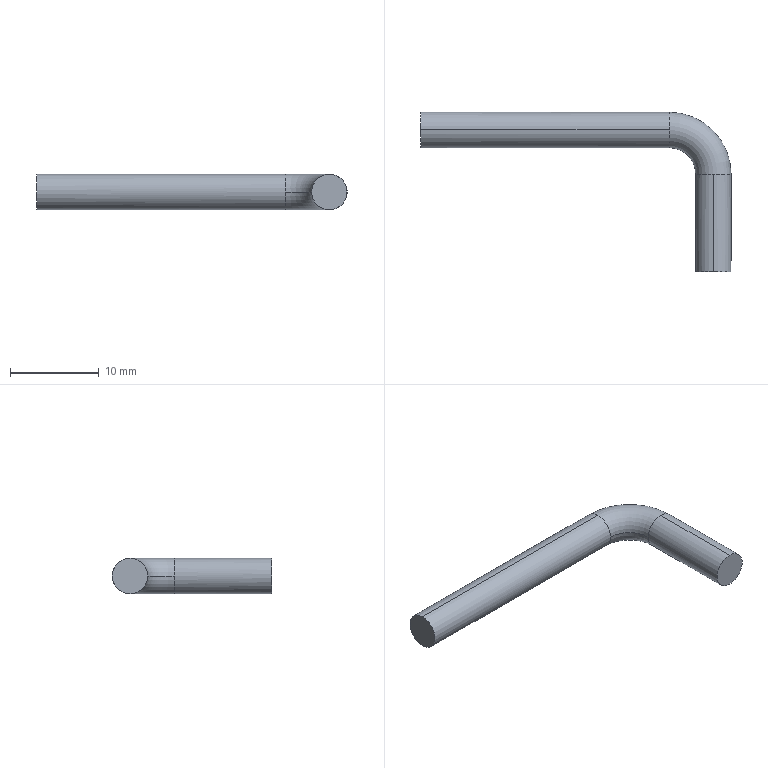Part | SolidWorks | features Sweep 1 | 1 solid | 8 faces | box 35 x 18 x 4 mm | volume 588.784 mm3 | cylinder 4 | torus 2 | plane 2 | commonest cylinder face diameters 4 x4
STEP:
#1=CARTESIAN_POINT('',(28.,2.,0.));
#2=VERTEX_POINT('',#1);
#3=CARTESIAN_POINT('',(28.,0.,-2.));
#4=VERTEX_POINT('',#3);
#5=CARTESIAN_POINT('',(28.,0.,0.));
#6=DIRECTION('',(-1.,0.,0.));
#7=DIRECTION('',(0.,0.,1.));
#8=AXIS2_PLACEMENT_3D('',#5,#6,#7);
#9=CIRCLE('',#8,2.);
#10=EDGE_CURVE('',#2,#4,#9,.T.);
#11=ORIENTED_EDGE('',*,*,#10,.F.);
#12=CARTESIAN_POINT('',(35.,-5.,0.));
#13=VERTEX_POINT('',#12);
#14=CARTESIAN_POINT('',(28.,-5.,0.));
#15=DIRECTION('',(0.,0.,-1.));
#16=DIRECTION('',(-1.,0.,0.));
#17=AXIS2_PLACEMENT_3D('',#14,#15,#16);
#18=CIRCLE('',#17,7.);
#19=EDGE_CURVE('',#2,#13,#18,.T.);
#20=ORIENTED_EDGE('',*,*,#19,.T.);
#21=CARTESIAN_POINT('',(33.,-5.,-2.));
#22=VERTEX_POINT('',#21);
#23=CARTESIAN_POINT('',(33.,-5.,0.));
#24=DIRECTION('',(0.,1.,0.));
#25=DIRECTION('',(0.,0.,1.));
#26=AXIS2_PLACEMENT_3D('',#23,#24,#25);
#27=CIRCLE('',#26,2.);
#28=EDGE_CURVE('',#13,#22,#27,.T.);
#29=ORIENTED_EDGE('',*,*,#28,.T.);
#30=CARTESIAN_POINT('',(31.,-5.,0.));
#31=VERTEX_POINT('',#30);
#32=CARTESIAN_POINT('',(33.,-5.,0.));
#33=DIRECTION('',(0.,1.,0.));
#34=DIRECTION('',(0.,0.,1.));
#35=AXIS2_PLACEMENT_3D('',#32,#33,#34);
#36=CIRCLE('',#35,2.);
#37=EDGE_CURVE('',#22,#31,#36,.T.);
#38=ORIENTED_EDGE('',*,*,#37,.T.);
#39=CARTESIAN_POINT('',(28.,-2.,0.));
#40=VERTEX_POINT('',#39);
#41=CARTESIAN_POINT('',(28.,-5.,0.));
#42=DIRECTION('',(0.,0.,-1.));
#43=DIRECTION('',(-1.,0.,0.));
#44=AXIS2_PLACEMENT_3D('',#41,#42,#43);
#45=CIRCLE('',#44,3.);
#46=EDGE_CURVE('',#40,#31,#45,.T.);
#47=ORIENTED_EDGE('',*,*,#46,.F.);
#48=CARTESIAN_POINT('',(28.,0.,0.));
#49=DIRECTION('',(-1.,0.,0.));
#50=DIRECTION('',(0.,0.,1.));
#51=AXIS2_PLACEMENT_3D('',#48,#49,#50);
#52=CIRCLE('',#51,2.);
#53=EDGE_CURVE('',#4,#40,#52,.T.);
#54=ORIENTED_EDGE('',*,*,#53,.F.);
#55=EDGE_LOOP('',(#11,#20,#29,#38,#47,#54));
#56=FACE_OUTER_BOUND('',#55,.T.);
#57=CARTESIAN_POINT('',(28.,-5.,0.));
#58=DIRECTION('',(0.,0.,-1.));
#59=DIRECTION('',(-1.,0.,0.));
#60=AXIS2_PLACEMENT_3D('',#57,#58,#59);
#61=TOROIDAL_SURFACE('',#60,5.,2.);
#62=ADVANCED_FACE('',(#56),#61,.T.);
#63=CARTESIAN_POINT('',(33.,-5.,2.));
#64=VERTEX_POINT('',#63);
#65=CARTESIAN_POINT('',(33.,-5.,0.));
#66=DIRECTION('',(0.,1.,0.));
#67=DIRECTION('',(0.,0.,1.));
#68=AXIS2_PLACEMENT_3D('',#65,#66,#67);
#69=CIRCLE('',#68,2.);
#70=EDGE_CURVE('',#64,#13,#69,.T.);
#71=ORIENTED_EDGE('',*,*,#70,.F.);
#72=CARTESIAN_POINT('',(33.,-16.,2.));
#73=VERTEX_POINT('',#72);
#74=CARTESIAN_POINT('',(33.,-5.,2.));
#75=DIRECTION('',(0.,-1.,0.));
#76=VECTOR('',#75,1000.);
#77=LINE('',#74,#76);
#78=EDGE_CURVE('',#64,#73,#77,.T.);
#79=ORIENTED_EDGE('',*,*,#78,.T.);
#80=CARTESIAN_POINT('',(33.,-16.,-2.));
#81=VERTEX_POINT('',#80);
#82=CARTESIAN_POINT('',(33.,-16.,0.));
#83=DIRECTION('',(0.,1.,0.));
#84=DIRECTION('',(0.,0.,1.));
#85=AXIS2_PLACEMENT_3D('',#82,#83,#84);
#86=CIRCLE('',#85,2.);
#87=EDGE_CURVE('',#73,#81,#86,.T.);
#88=ORIENTED_EDGE('',*,*,#87,.T.);
#89=CARTESIAN_POINT('',(33.,-5.,-2.));
#90=DIRECTION('',(0.,-1.,0.));
#91=VECTOR('',#90,1000.);
#92=LINE('',#89,#91);
#93=EDGE_CURVE('',#22,#81,#92,.T.);
#94=ORIENTED_EDGE('',*,*,#93,.F.);
#95=ORIENTED_EDGE('',*,*,#28,.F.);
#96=EDGE_LOOP('',(#71,#79,#88,#94,#95));
#97=FACE_OUTER_BOUND('',#96,.T.);
#98=CARTESIAN_POINT('',(33.,-5.,0.));
#99=DIRECTION('',(0.,-1.,0.));
#100=DIRECTION('',(0.,0.,-1.));
#101=AXIS2_PLACEMENT_3D('',#98,#99,#100);
#102=CYLINDRICAL_SURFACE('',#101,2.);
#103=ADVANCED_FACE('',(#97),#102,.T.);
#104=CARTESIAN_POINT('',(0.,0.,2.));
#105=VERTEX_POINT('',#104);
#106=CARTESIAN_POINT('',(0.,0.,-2.));
#107=VERTEX_POINT('',#106);
#108=CARTESIAN_POINT('',(0.,0.,0.));
#109=DIRECTION('',(-1.,0.,0.));
#110=DIRECTION('',(0.,0.,1.));
#111=AXIS2_PLACEMENT_3D('',#108,#109,#110);
#112=CIRCLE('',#111,2.);
#113=EDGE_CURVE('',#105,#107,#112,.T.);
#114=ORIENTED_EDGE('',*,*,#113,.F.);
#115=CARTESIAN_POINT('',(28.,0.,2.));
#116=VERTEX_POINT('',#115);
#117=CARTESIAN_POINT('',(0.,0.,2.));
#118=DIRECTION('',(1.,0.,0.));
#119=VECTOR('',#118,1000.);
#120=LINE('',#117,#119);
#121=EDGE_CURVE('',#105,#116,#120,.T.);
#122=ORIENTED_EDGE('',*,*,#121,.T.);
#123=CARTESIAN_POINT('',(28.,0.,0.));
#124=DIRECTION('',(-1.,0.,0.));
#125=DIRECTION('',(0.,0.,1.));
#126=AXIS2_PLACEMENT_3D('',#123,#124,#125);
#127=CIRCLE('',#126,2.);
#128=EDGE_CURVE('',#116,#2,#127,.T.);
#129=ORIENTED_EDGE('',*,*,#128,.T.);
#130=ORIENTED_EDGE('',*,*,#10,.T.);
#131=CARTESIAN_POINT('',(0.,0.,-2.));
#132=DIRECTION('',(1.,0.,0.));
#133=VECTOR('',#132,1000.);
#134=LINE('',#131,#133);
#135=EDGE_CURVE('',#107,#4,#134,.T.);
#136=ORIENTED_EDGE('',*,*,#135,.F.);
#137=EDGE_LOOP('',(#114,#122,#129,#130,#136));
#138=FACE_OUTER_BOUND('',#137,.T.);
#139=CARTESIAN_POINT('',(0.,0.,0.));
#140=DIRECTION('',(1.,0.,0.));
#141=DIRECTION('',(0.,0.,-1.));
#142=AXIS2_PLACEMENT_3D('',#139,#140,#141);
#143=CYLINDRICAL_SURFACE('',#142,2.);
#144=ADVANCED_FACE('',(#138),#143,.T.);
#145=ORIENTED_EDGE('',*,*,#78,.F.);
#146=CARTESIAN_POINT('',(33.,-5.,0.));
#147=DIRECTION('',(0.,1.,0.));
#148=DIRECTION('',(0.,0.,1.));
#149=AXIS2_PLACEMENT_3D('',#146,#147,#148);
#150=CIRCLE('',#149,2.);
#151=EDGE_CURVE('',#31,#64,#150,.T.);
#152=ORIENTED_EDGE('',*,*,#151,.F.);
#153=ORIENTED_EDGE('',*,*,#37,.F.);
#154=ORIENTED_EDGE('',*,*,#93,.T.);
#155=CARTESIAN_POINT('',(33.,-16.,0.));
#156=DIRECTION('',(0.,1.,0.));
#157=DIRECTION('',(0.,0.,1.));
#158=AXIS2_PLACEMENT_3D('',#155,#156,#157);
#159=CIRCLE('',#158,2.);
#160=EDGE_CURVE('',#81,#73,#159,.T.);
#161=ORIENTED_EDGE('',*,*,#160,.T.);
#162=EDGE_LOOP('',(#145,#152,#153,#154,#161));
#163=FACE_OUTER_BOUND('',#162,.T.);
#164=CARTESIAN_POINT('',(33.,-5.,0.));
#165=DIRECTION('',(0.,-1.,0.));
#166=DIRECTION('',(0.,0.,-1.));
#167=AXIS2_PLACEMENT_3D('',#164,#165,#166);
#168=CYLINDRICAL_SURFACE('',#167,2.);
#169=ADVANCED_FACE('',(#163),#168,.T.);
#170=ORIENTED_EDGE('',*,*,#19,.F.);
#171=ORIENTED_EDGE('',*,*,#128,.F.);
#172=CARTESIAN_POINT('',(28.,0.,0.));
#173=DIRECTION('',(-1.,0.,0.));
#174=DIRECTION('',(0.,0.,1.));
#175=AXIS2_PLACEMENT_3D('',#172,#173,#174);
#176=CIRCLE('',#175,2.);
#177=EDGE_CURVE('',#40,#116,#176,.T.);
#178=ORIENTED_EDGE('',*,*,#177,.F.);
#179=ORIENTED_EDGE('',*,*,#46,.T.);
#180=ORIENTED_EDGE('',*,*,#151,.T.);
#181=ORIENTED_EDGE('',*,*,#70,.T.);
#182=EDGE_LOOP('',(#170,#171,#178,#179,#180,#181));
#183=FACE_OUTER_BOUND('',#182,.T.);
#184=CARTESIAN_POINT('',(28.,-5.,0.));
#185=DIRECTION('',(0.,0.,-1.));
#186=DIRECTION('',(-1.,0.,0.));
#187=AXIS2_PLACEMENT_3D('',#184,#185,#186);
#188=TOROIDAL_SURFACE('',#187,5.,2.);
#189=ADVANCED_FACE('',(#183),#188,.T.);
#190=ORIENTED_EDGE('',*,*,#121,.F.);
#191=CARTESIAN_POINT('',(0.,0.,0.));
#192=DIRECTION('',(-1.,0.,0.));
#193=DIRECTION('',(0.,0.,1.));
#194=AXIS2_PLACEMENT_3D('',#191,#192,#193);
#195=CIRCLE('',#194,2.);
#196=EDGE_CURVE('',#107,#105,#195,.T.);
#197=ORIENTED_EDGE('',*,*,#196,.F.);
#198=ORIENTED_EDGE('',*,*,#135,.T.);
#199=ORIENTED_EDGE('',*,*,#53,.T.);
#200=ORIENTED_EDGE('',*,*,#177,.T.);
#201=EDGE_LOOP('',(#190,#197,#198,#199,#200));
#202=FACE_OUTER_BOUND('',#201,.T.);
#203=CARTESIAN_POINT('',(0.,0.,0.));
#204=DIRECTION('',(1.,0.,0.));
#205=DIRECTION('',(0.,0.,-1.));
#206=AXIS2_PLACEMENT_3D('',#203,#204,#205);
#207=CYLINDRICAL_SURFACE('',#206,2.);
#208=ADVANCED_FACE('',(#202),#207,.T.);
#209=ORIENTED_EDGE('',*,*,#160,.F.);
#210=ORIENTED_EDGE('',*,*,#87,.F.);
#211=EDGE_LOOP('',(#209,#210));
#212=FACE_OUTER_BOUND('',#211,.T.);
#213=CARTESIAN_POINT('',(33.,-16.,0.));
#214=DIRECTION('',(0.,1.,0.));
#215=DIRECTION('',(0.,0.,1.));
#216=AXIS2_PLACEMENT_3D('',#213,#214,#215);
#217=PLANE('',#216);
#218=ADVANCED_FACE('',(#212),#217,.F.);
#219=ORIENTED_EDGE('',*,*,#196,.T.);
#220=ORIENTED_EDGE('',*,*,#113,.T.);
#221=EDGE_LOOP('',(#219,#220));
#222=FACE_OUTER_BOUND('',#221,.T.);
#223=CARTESIAN_POINT('',(0.,0.,0.));
#224=DIRECTION('',(-1.,0.,0.));
#225=DIRECTION('',(0.,0.,1.));
#226=AXIS2_PLACEMENT_3D('',#223,#224,#225);
#227=PLANE('',#226);
#228=ADVANCED_FACE('',(#222),#227,.T.);
#229=CLOSED_SHELL('',(#62,#103,#144,#169,#189,#208,#218,#228));
#230=MANIFOLD_SOLID_BREP('',#229);
#231=CARTESIAN_POINT('',(0.,0.,0.));
#232=DIRECTION('',(0.,0.,1.));
#233=DIRECTION('',(1.,0.,0.));
#234=AXIS2_PLACEMENT_3D('',#231,#232,#233);
#235=(LENGTH_UNIT()NAMED_UNIT(*)SI_UNIT(.MILLI.,.METRE.));
#236=UNCERTAINTY_MEASURE_WITH_UNIT(LENGTH_MEASURE(0.00001),#235,'','');
#237=(NAMED_UNIT(*)PLANE_ANGLE_UNIT()SI_UNIT($,.RADIAN.));
#238=(NAMED_UNIT(*)SI_UNIT($,.STERADIAN.)SOLID_ANGLE_UNIT());
#239=(GEOMETRIC_REPRESENTATION_CONTEXT(3)GLOBAL_UNCERTAINTY_ASSIGNED_CONTEXT((#236))GLOBAL_UNIT_ASSIGNED_CONTEXT((#235,#237,#238))REPRESENTATION_CONTEXT('',''));
#240=ADVANCED_BREP_SHAPE_REPRESENTATION('',(#230,#234),#239);